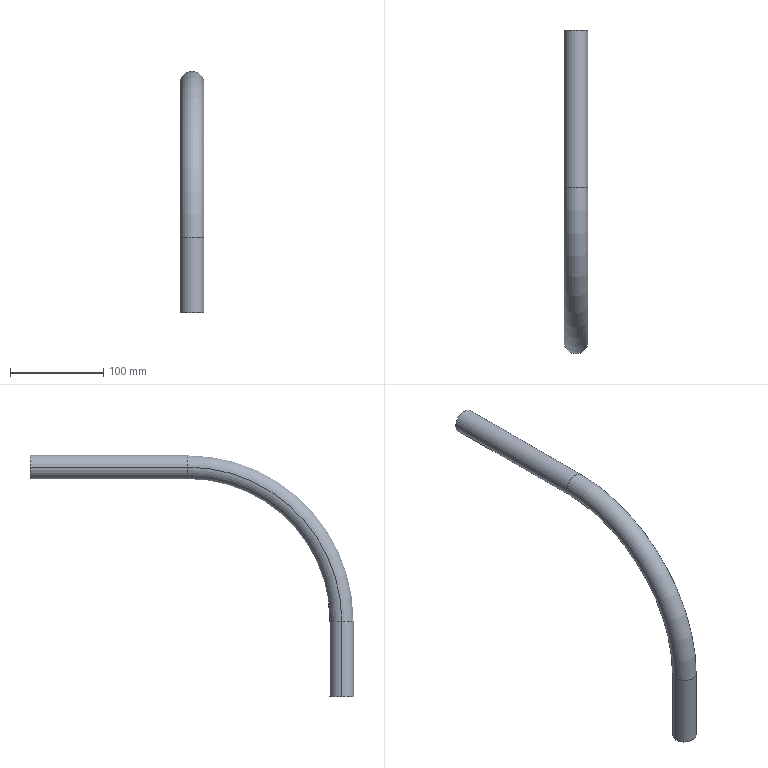Part | STEP file | 31E-01144WG10 | 1 solid | 17 faces | box 25.4 x 346.08 x 258.41 mm | volume 96204 mm3 | cylinder 10 | torus 4 | plane 3 | commonest cylinder face diameters 19.8 x4 25.4 x4 23 x2
STEP:
#1=CARTESIAN_POINT('',(-12.7,-168.38,0.));
#2=VERTEX_POINT('',#1);
#3=CARTESIAN_POINT('',(12.7,-168.38,0.));
#4=VERTEX_POINT('',#3);
#5=CARTESIAN_POINT('',(0.,-168.38,0.));
#6=DIRECTION('',(0.,1.,0.));
#7=AXIS2_PLACEMENT_3D('',#5,#6,$);
#8=CIRCLE('',#7,12.7);
#9=EDGE_CURVE('',#2,#4,#8,.T.);
#10=ORIENTED_EDGE('',*,*,#9,.T.);
#11=CARTESIAN_POINT('',(12.7,0.,0.));
#12=VERTEX_POINT('',#11);
#13=CARTESIAN_POINT('',(12.7,-84.19,0.));
#14=DIRECTION('',(0.,1.,0.));
#15=VECTOR('',#14,1.);
#16=LINE('',#13,#15);
#17=EDGE_CURVE('',#12,#4,#16,.F.);
#18=ORIENTED_EDGE('',*,*,#17,.F.);
#19=CARTESIAN_POINT('',(-12.7,0.,0.));
#20=VERTEX_POINT('',#19);
#21=CARTESIAN_POINT('',(0.,0.,0.));
#22=DIRECTION('',(0.,1.,0.));
#23=AXIS2_PLACEMENT_3D('',#21,#22,$);
#24=CIRCLE('',#23,12.7);
#25=EDGE_CURVE('',#20,#12,#24,.T.);
#26=ORIENTED_EDGE('',*,*,#25,.F.);
#27=CARTESIAN_POINT('',(-12.7,-84.19,0.));
#28=DIRECTION('',(0.,1.,0.));
#29=VECTOR('',#28,1.);
#30=LINE('',#27,#29);
#31=EDGE_CURVE('',#20,#2,#30,.F.);
#32=ORIENTED_EDGE('',*,*,#31,.T.);
#33=EDGE_LOOP('',(#10,#18,#26,#32));
#34=FACE_OUTER_BOUND('',#33,.T.);
#35=CARTESIAN_POINT('',(0.,-84.19,0.));
#36=DIRECTION('',(0.,1.,0.));
#37=DIRECTION('',(-1.,0.,0.));
#38=AXIS2_PLACEMENT_3D('',#35,#36,#37);
#39=CYLINDRICAL_SURFACE('',#38,12.7);
#40=ADVANCED_FACE('',(#34),#39,.T.);
#41=CARTESIAN_POINT('',(0.,-168.38,0.));
#42=DIRECTION('',(0.,1.,0.));
#43=AXIS2_PLACEMENT_3D('',#41,#42,$);
#44=CIRCLE('',#43,12.7);
#45=EDGE_CURVE('',#4,#2,#44,.T.);
#46=ORIENTED_EDGE('',*,*,#45,.T.);
#47=ORIENTED_EDGE('',*,*,#31,.F.);
#48=CARTESIAN_POINT('',(0.,0.,0.));
#49=DIRECTION('',(0.,1.,0.));
#50=AXIS2_PLACEMENT_3D('',#48,#49,$);
#51=CIRCLE('',#50,12.7);
#52=EDGE_CURVE('',#12,#20,#51,.T.);
#53=ORIENTED_EDGE('',*,*,#52,.F.);
#54=ORIENTED_EDGE('',*,*,#17,.T.);
#55=EDGE_LOOP('',(#46,#47,#53,#54));
#56=FACE_OUTER_BOUND('',#55,.T.);
#57=CARTESIAN_POINT('',(0.,-84.19,0.));
#58=DIRECTION('',(0.,1.,0.));
#59=DIRECTION('',(1.,0.,0.));
#60=AXIS2_PLACEMENT_3D('',#57,#58,#59);
#61=CYLINDRICAL_SURFACE('',#60,12.7);
#62=ADVANCED_FACE('',(#56),#61,.T.);
#63=CARTESIAN_POINT('',(-12.7,-333.38,-165.));
#64=VERTEX_POINT('',#63);
#65=CARTESIAN_POINT('',(12.7,-333.38,-165.));
#66=VERTEX_POINT('',#65);
#67=CARTESIAN_POINT('',(0.,-333.38,-165.));
#68=DIRECTION('',(0.,0.,1.));
#69=AXIS2_PLACEMENT_3D('',#67,#68,$);
#70=CIRCLE('',#69,12.7);
#71=EDGE_CURVE('',#64,#66,#70,.T.);
#72=ORIENTED_EDGE('',*,*,#71,.T.);
#73=CARTESIAN_POINT('',(12.7,-168.38,-165.));
#74=DIRECTION('',(1.,0.,0.));
#75=AXIS2_PLACEMENT_3D('',#73,#74,$);
#76=CIRCLE('',#75,165.);
#77=EDGE_CURVE('',#4,#66,#76,.T.);
#78=ORIENTED_EDGE('',*,*,#77,.F.);
#79=ORIENTED_EDGE('',*,*,#9,.F.);
#80=CARTESIAN_POINT('',(-12.7,-168.38,-165.));
#81=DIRECTION('',(1.,0.,0.));
#82=AXIS2_PLACEMENT_3D('',#80,#81,$);
#83=CIRCLE('',#82,165.);
#84=EDGE_CURVE('',#2,#64,#83,.T.);
#85=ORIENTED_EDGE('',*,*,#84,.T.);
#86=EDGE_LOOP('',(#72,#78,#79,#85));
#87=FACE_OUTER_BOUND('',#86,.T.);
#88=CARTESIAN_POINT('',(0.,-168.38,-165.));
#89=DIRECTION('',(1.,0.,0.));
#90=DIRECTION('',(0.,0.,1.));
#91=AXIS2_PLACEMENT_3D('',#88,#89,#90);
#92=TOROIDAL_SURFACE('',#91,165.,12.7);
#93=ADVANCED_FACE('',(#87),#92,.T.);
#94=CARTESIAN_POINT('',(0.,-333.38,-165.));
#95=DIRECTION('',(0.,0.,1.));
#96=AXIS2_PLACEMENT_3D('',#94,#95,$);
#97=CIRCLE('',#96,12.7);
#98=EDGE_CURVE('',#66,#64,#97,.T.);
#99=ORIENTED_EDGE('',*,*,#98,.T.);
#100=ORIENTED_EDGE('',*,*,#84,.F.);
#101=ORIENTED_EDGE('',*,*,#45,.F.);
#102=ORIENTED_EDGE('',*,*,#77,.T.);
#103=EDGE_LOOP('',(#99,#100,#101,#102));
#104=FACE_OUTER_BOUND('',#103,.T.);
#105=CARTESIAN_POINT('',(0.,-168.38,-165.));
#106=DIRECTION('',(1.,0.,0.));
#107=DIRECTION('',(0.,0.,1.));
#108=AXIS2_PLACEMENT_3D('',#105,#106,#107);
#109=TOROIDAL_SURFACE('',#108,165.,12.7);
#110=ADVANCED_FACE('',(#104),#109,.T.);
#111=CARTESIAN_POINT('',(-12.7,-333.38,-245.71));
#112=VERTEX_POINT('',#111);
#113=CARTESIAN_POINT('',(12.7,-333.38,-245.71));
#114=VERTEX_POINT('',#113);
#115=CARTESIAN_POINT('',(0.,-333.38,-245.71));
#116=DIRECTION('',(0.,0.,1.));
#117=AXIS2_PLACEMENT_3D('',#115,#116,$);
#118=CIRCLE('',#117,12.7);
#119=EDGE_CURVE('',#112,#114,#118,.T.);
#120=ORIENTED_EDGE('',*,*,#119,.T.);
#121=CARTESIAN_POINT('',(12.7,-333.38,-205.355));
#122=DIRECTION('',(0.,0.,1.));
#123=VECTOR('',#122,1.);
#124=LINE('',#121,#123);
#125=EDGE_CURVE('',#66,#114,#124,.F.);
#126=ORIENTED_EDGE('',*,*,#125,.F.);
#127=ORIENTED_EDGE('',*,*,#71,.F.);
#128=CARTESIAN_POINT('',(-12.7,-333.38,-205.355));
#129=DIRECTION('',(0.,0.,1.));
#130=VECTOR('',#129,1.);
#131=LINE('',#128,#130);
#132=EDGE_CURVE('',#64,#112,#131,.F.);
#133=ORIENTED_EDGE('',*,*,#132,.T.);
#134=EDGE_LOOP('',(#120,#126,#127,#133));
#135=FACE_OUTER_BOUND('',#134,.T.);
#136=CARTESIAN_POINT('',(0.,-333.38,-205.355));
#137=DIRECTION('',(0.,0.,1.));
#138=DIRECTION('',(-1.,0.,0.));
#139=AXIS2_PLACEMENT_3D('',#136,#137,#138);
#140=CYLINDRICAL_SURFACE('',#139,12.7);
#141=ADVANCED_FACE('',(#135),#140,.T.);
#142=CARTESIAN_POINT('',(0.,-333.38,-245.71));
#143=DIRECTION('',(0.,0.,1.));
#144=AXIS2_PLACEMENT_3D('',#142,#143,$);
#145=CIRCLE('',#144,12.7);
#146=EDGE_CURVE('',#114,#112,#145,.T.);
#147=ORIENTED_EDGE('',*,*,#146,.T.);
#148=ORIENTED_EDGE('',*,*,#132,.F.);
#149=ORIENTED_EDGE('',*,*,#98,.F.);
#150=ORIENTED_EDGE('',*,*,#125,.T.);
#151=EDGE_LOOP('',(#147,#148,#149,#150));
#152=FACE_OUTER_BOUND('',#151,.T.);
#153=CARTESIAN_POINT('',(0.,-333.38,-205.355));
#154=DIRECTION('',(0.,0.,1.));
#155=DIRECTION('',(1.,0.,0.));
#156=AXIS2_PLACEMENT_3D('',#153,#154,#155);
#157=CYLINDRICAL_SURFACE('',#156,12.7);
#158=ADVANCED_FACE('',(#152),#157,.T.);
#159=CARTESIAN_POINT('',(-9.9,-168.38,0.));
#160=VERTEX_POINT('',#159);
#161=CARTESIAN_POINT('',(-9.9,-333.38,-165.));
#162=VERTEX_POINT('',#161);
#163=CARTESIAN_POINT('',(-9.9,-168.38,-165.));
#164=DIRECTION('',(1.,0.,0.));
#165=AXIS2_PLACEMENT_3D('',#163,#164,$);
#166=CIRCLE('',#165,165.);
#167=EDGE_CURVE('',#160,#162,#166,.T.);
#168=ORIENTED_EDGE('',*,*,#167,.F.);
#169=CARTESIAN_POINT('',(9.9,-168.38,0.));
#170=VERTEX_POINT('',#169);
#171=CARTESIAN_POINT('',(0.,-168.38,0.));
#172=DIRECTION('',(0.,1.,0.));
#173=AXIS2_PLACEMENT_3D('',#171,#172,$);
#174=CIRCLE('',#173,9.9);
#175=EDGE_CURVE('',#160,#170,#174,.T.);
#176=ORIENTED_EDGE('',*,*,#175,.T.);
#177=CARTESIAN_POINT('',(9.9,-333.38,-165.));
#178=VERTEX_POINT('',#177);
#179=CARTESIAN_POINT('',(9.9,-168.38,-165.));
#180=DIRECTION('',(1.,0.,0.));
#181=AXIS2_PLACEMENT_3D('',#179,#180,$);
#182=CIRCLE('',#181,165.);
#183=EDGE_CURVE('',#170,#178,#182,.T.);
#184=ORIENTED_EDGE('',*,*,#183,.T.);
#185=CARTESIAN_POINT('',(0.,-333.38,-165.));
#186=DIRECTION('',(0.,0.,1.));
#187=AXIS2_PLACEMENT_3D('',#185,#186,$);
#188=CIRCLE('',#187,9.9);
#189=EDGE_CURVE('',#162,#178,#188,.T.);
#190=ORIENTED_EDGE('',*,*,#189,.F.);
#191=EDGE_LOOP('',(#168,#176,#184,#190));
#192=FACE_OUTER_BOUND('',#191,.T.);
#193=CARTESIAN_POINT('',(0.,-168.38,-165.));
#194=DIRECTION('',(1.,0.,0.));
#195=DIRECTION('',(0.,0.,1.));
#196=AXIS2_PLACEMENT_3D('',#193,#194,#195);
#197=TOROIDAL_SURFACE('',#196,165.,9.9);
#198=ADVANCED_FACE('',(#192),#197,.F.);
#199=ORIENTED_EDGE('',*,*,#183,.F.);
#200=CARTESIAN_POINT('',(0.,-168.38,0.));
#201=DIRECTION('',(0.,1.,0.));
#202=AXIS2_PLACEMENT_3D('',#200,#201,$);
#203=CIRCLE('',#202,9.9);
#204=EDGE_CURVE('',#170,#160,#203,.T.);
#205=ORIENTED_EDGE('',*,*,#204,.T.);
#206=ORIENTED_EDGE('',*,*,#167,.T.);
#207=CARTESIAN_POINT('',(0.,-333.38,-165.));
#208=DIRECTION('',(0.,0.,1.));
#209=AXIS2_PLACEMENT_3D('',#207,#208,$);
#210=CIRCLE('',#209,9.9);
#211=EDGE_CURVE('',#178,#162,#210,.T.);
#212=ORIENTED_EDGE('',*,*,#211,.F.);
#213=EDGE_LOOP('',(#199,#205,#206,#212));
#214=FACE_OUTER_BOUND('',#213,.T.);
#215=CARTESIAN_POINT('',(0.,-168.38,-165.));
#216=DIRECTION('',(1.,0.,0.));
#217=DIRECTION('',(0.,0.,1.));
#218=AXIS2_PLACEMENT_3D('',#215,#216,#217);
#219=TOROIDAL_SURFACE('',#218,165.,9.9);
#220=ADVANCED_FACE('',(#214),#219,.F.);
#221=ORIENTED_EDGE('',*,*,#146,.F.);
#222=ORIENTED_EDGE('',*,*,#119,.F.);
#223=EDGE_LOOP('',(#221,#222));
#224=FACE_OUTER_BOUND('',#223,.T.);
#225=CARTESIAN_POINT('',(9.9,-333.38,-245.71));
#226=VERTEX_POINT('',#225);
#227=CARTESIAN_POINT('',(-9.9,-333.38,-245.71));
#228=VERTEX_POINT('',#227);
#229=CARTESIAN_POINT('',(0.,-333.38,-245.71));
#230=DIRECTION('',(0.,0.,-1.));
#231=AXIS2_PLACEMENT_3D('',#229,#230,$);
#232=CIRCLE('',#231,9.9);
#233=EDGE_CURVE('',#226,#228,#232,.F.);
#234=ORIENTED_EDGE('',*,*,#233,.T.);
#235=CARTESIAN_POINT('',(0.,-333.38,-245.71));
#236=DIRECTION('',(0.,0.,-1.));
#237=AXIS2_PLACEMENT_3D('',#235,#236,$);
#238=CIRCLE('',#237,9.9);
#239=EDGE_CURVE('',#228,#226,#238,.F.);
#240=ORIENTED_EDGE('',*,*,#239,.T.);
#241=EDGE_LOOP('',(#234,#240));
#242=FACE_BOUND('',#241,.T.);
#243=CARTESIAN_POINT('',(0.,-333.38,-245.71));
#244=DIRECTION('',(0.,0.,-1.));
#245=DIRECTION('',(0.,1.,0.));
#246=AXIS2_PLACEMENT_3D('',#243,#244,#245);
#247=PLANE('',#246);
#248=ADVANCED_FACE('',(#224,#242),#247,.T.);
#249=CARTESIAN_POINT('',(-9.9,-333.38,-205.355));
#250=DIRECTION('',(0.,0.,1.));
#251=VECTOR('',#250,1.);
#252=LINE('',#249,#251);
#253=EDGE_CURVE('',#162,#228,#252,.F.);
#254=ORIENTED_EDGE('',*,*,#253,.F.);
#255=ORIENTED_EDGE('',*,*,#189,.T.);
#256=CARTESIAN_POINT('',(9.9,-333.38,-205.355));
#257=DIRECTION('',(0.,0.,1.));
#258=VECTOR('',#257,1.);
#259=LINE('',#256,#258);
#260=EDGE_CURVE('',#178,#226,#259,.F.);
#261=ORIENTED_EDGE('',*,*,#260,.T.);
#262=ORIENTED_EDGE('',*,*,#239,.F.);
#263=EDGE_LOOP('',(#254,#255,#261,#262));
#264=FACE_OUTER_BOUND('',#263,.T.);
#265=CARTESIAN_POINT('',(0.,-333.38,-205.355));
#266=DIRECTION('',(0.,0.,1.));
#267=DIRECTION('',(-1.,0.,0.));
#268=AXIS2_PLACEMENT_3D('',#265,#266,#267);
#269=CYLINDRICAL_SURFACE('',#268,9.9);
#270=ADVANCED_FACE('',(#264),#269,.F.);
#271=ORIENTED_EDGE('',*,*,#260,.F.);
#272=ORIENTED_EDGE('',*,*,#211,.T.);
#273=ORIENTED_EDGE('',*,*,#253,.T.);
#274=ORIENTED_EDGE('',*,*,#233,.F.);
#275=EDGE_LOOP('',(#271,#272,#273,#274));
#276=FACE_OUTER_BOUND('',#275,.T.);
#277=CARTESIAN_POINT('',(0.,-333.38,-205.355));
#278=DIRECTION('',(0.,0.,1.));
#279=DIRECTION('',(1.,0.,0.));
#280=AXIS2_PLACEMENT_3D('',#277,#278,#279);
#281=CYLINDRICAL_SURFACE('',#280,9.9);
#282=ADVANCED_FACE('',(#276),#281,.F.);
#283=CARTESIAN_POINT('',(9.9,-45.,0.));
#284=VERTEX_POINT('',#283);
#285=CARTESIAN_POINT('',(-9.9,-45.,0.));
#286=VERTEX_POINT('',#285);
#287=CARTESIAN_POINT('',(0.,-45.,0.));
#288=DIRECTION('',(0.,1.,0.));
#289=AXIS2_PLACEMENT_3D('',#287,#288,$);
#290=CIRCLE('',#289,9.9);
#291=EDGE_CURVE('',#284,#286,#290,.T.);
#292=ORIENTED_EDGE('',*,*,#291,.T.);
#293=CARTESIAN_POINT('',(-9.9,-84.19,0.));
#294=DIRECTION('',(0.,1.,0.));
#295=VECTOR('',#294,1.);
#296=LINE('',#293,#295);
#297=EDGE_CURVE('',#286,#160,#296,.F.);
#298=ORIENTED_EDGE('',*,*,#297,.T.);
#299=ORIENTED_EDGE('',*,*,#204,.F.);
#300=CARTESIAN_POINT('',(9.9,-84.19,0.));
#301=DIRECTION('',(0.,1.,0.));
#302=VECTOR('',#301,1.);
#303=LINE('',#300,#302);
#304=EDGE_CURVE('',#284,#170,#303,.F.);
#305=ORIENTED_EDGE('',*,*,#304,.F.);
#306=EDGE_LOOP('',(#292,#298,#299,#305));
#307=FACE_OUTER_BOUND('',#306,.T.);
#308=CARTESIAN_POINT('',(0.,-84.19,0.));
#309=DIRECTION('',(0.,1.,0.));
#310=DIRECTION('',(1.,0.,0.));
#311=AXIS2_PLACEMENT_3D('',#308,#309,#310);
#312=CYLINDRICAL_SURFACE('',#311,9.9);
#313=ADVANCED_FACE('',(#307),#312,.F.);
#314=CARTESIAN_POINT('',(0.,-45.,0.));
#315=DIRECTION('',(0.,1.,0.));
#316=AXIS2_PLACEMENT_3D('',#314,#315,$);
#317=CIRCLE('',#316,9.9);
#318=EDGE_CURVE('',#286,#284,#317,.T.);
#319=ORIENTED_EDGE('',*,*,#318,.T.);
#320=ORIENTED_EDGE('',*,*,#304,.T.);
#321=ORIENTED_EDGE('',*,*,#175,.F.);
#322=ORIENTED_EDGE('',*,*,#297,.F.);
#323=EDGE_LOOP('',(#319,#320,#321,#322));
#324=FACE_OUTER_BOUND('',#323,.T.);
#325=CARTESIAN_POINT('',(0.,-84.19,0.));
#326=DIRECTION('',(0.,1.,0.));
#327=DIRECTION('',(-1.,0.,0.));
#328=AXIS2_PLACEMENT_3D('',#325,#326,#327);
#329=CYLINDRICAL_SURFACE('',#328,9.9);
#330=ADVANCED_FACE('',(#324),#329,.F.);
#331=ORIENTED_EDGE('',*,*,#25,.T.);
#332=ORIENTED_EDGE('',*,*,#52,.T.);
#333=EDGE_LOOP('',(#331,#332));
#334=FACE_OUTER_BOUND('',#333,.T.);
#335=CARTESIAN_POINT('',(-11.5,0.,0.));
#336=VERTEX_POINT('',#335);
#337=CARTESIAN_POINT('',(11.5,0.,0.));
#338=VERTEX_POINT('',#337);
#339=CARTESIAN_POINT('',(0.,0.,0.));
#340=DIRECTION('',(0.,1.,0.));
#341=AXIS2_PLACEMENT_3D('',#339,#340,$);
#342=CIRCLE('',#341,11.5);
#343=EDGE_CURVE('',#336,#338,#342,.T.);
#344=ORIENTED_EDGE('',*,*,#343,.F.);
#345=CARTESIAN_POINT('',(0.,0.,0.));
#346=DIRECTION('',(0.,1.,0.));
#347=AXIS2_PLACEMENT_3D('',#345,#346,$);
#348=CIRCLE('',#347,11.5);
#349=EDGE_CURVE('',#338,#336,#348,.T.);
#350=ORIENTED_EDGE('',*,*,#349,.F.);
#351=EDGE_LOOP('',(#344,#350));
#352=FACE_BOUND('',#351,.T.);
#353=CARTESIAN_POINT('',(0.,0.,0.));
#354=DIRECTION('',(0.,1.,0.));
#355=DIRECTION('',(0.,0.,1.));
#356=AXIS2_PLACEMENT_3D('',#353,#354,#355);
#357=PLANE('',#356);
#358=ADVANCED_FACE('',(#334,#352),#357,.T.);
#359=CARTESIAN_POINT('',(-11.5,-45.,0.));
#360=VERTEX_POINT('',#359);
#361=CARTESIAN_POINT('',(-11.5,-22.5,0.));
#362=DIRECTION('',(0.,1.,0.));
#363=VECTOR('',#362,1.);
#364=LINE('',#361,#363);
#365=EDGE_CURVE('',#336,#360,#364,.F.);
#366=ORIENTED_EDGE('',*,*,#365,.F.);
#367=ORIENTED_EDGE('',*,*,#343,.T.);
#368=CARTESIAN_POINT('',(11.5,-45.,0.));
#369=VERTEX_POINT('',#368);
#370=CARTESIAN_POINT('',(11.5,-22.5,0.));
#371=DIRECTION('',(0.,1.,0.));
#372=VECTOR('',#371,1.);
#373=LINE('',#370,#372);
#374=EDGE_CURVE('',#338,#369,#373,.F.);
#375=ORIENTED_EDGE('',*,*,#374,.T.);
#376=CARTESIAN_POINT('',(0.,-45.,0.));
#377=DIRECTION('',(0.,1.,0.));
#378=AXIS2_PLACEMENT_3D('',#376,#377,$);
#379=CIRCLE('',#378,11.5);
#380=EDGE_CURVE('',#360,#369,#379,.T.);
#381=ORIENTED_EDGE('',*,*,#380,.F.);
#382=EDGE_LOOP('',(#366,#367,#375,#381));
#383=FACE_OUTER_BOUND('',#382,.T.);
#384=CARTESIAN_POINT('',(0.,-22.5,0.));
#385=DIRECTION('',(0.,1.,0.));
#386=DIRECTION('',(-1.,0.,0.));
#387=AXIS2_PLACEMENT_3D('',#384,#385,#386);
#388=CYLINDRICAL_SURFACE('',#387,11.5);
#389=ADVANCED_FACE('',(#383),#388,.F.);
#390=ORIENTED_EDGE('',*,*,#374,.F.);
#391=ORIENTED_EDGE('',*,*,#349,.T.);
#392=ORIENTED_EDGE('',*,*,#365,.T.);
#393=CARTESIAN_POINT('',(0.,-45.,0.));
#394=DIRECTION('',(0.,1.,0.));
#395=AXIS2_PLACEMENT_3D('',#393,#394,$);
#396=CIRCLE('',#395,11.5);
#397=EDGE_CURVE('',#369,#360,#396,.T.);
#398=ORIENTED_EDGE('',*,*,#397,.F.);
#399=EDGE_LOOP('',(#390,#391,#392,#398));
#400=FACE_OUTER_BOUND('',#399,.T.);
#401=ADVANCED_FACE('',(#400),#388,.F.);
#402=ORIENTED_EDGE('',*,*,#380,.T.);
#403=ORIENTED_EDGE('',*,*,#397,.T.);
#404=EDGE_LOOP('',(#402,#403));
#405=FACE_OUTER_BOUND('',#404,.T.);
#406=ORIENTED_EDGE('',*,*,#318,.F.);
#407=ORIENTED_EDGE('',*,*,#291,.F.);
#408=EDGE_LOOP('',(#406,#407));
#409=FACE_BOUND('',#408,.T.);
#410=CARTESIAN_POINT('',(0.,-45.,0.));
#411=DIRECTION('',(0.,1.,0.));
#412=DIRECTION('',(-1.,0.,0.));
#413=AXIS2_PLACEMENT_3D('',#410,#411,#412);
#414=PLANE('',#413);
#415=ADVANCED_FACE('',(#405,#409),#414,.T.);
#416=CLOSED_SHELL('',(#40,#62,#93,#110,#141,#158,#198,#220,#248,#270,#282,#313,#330,#358,#389,#401,#415));
#417=MANIFOLD_SOLID_BREP('',#416);
#418=(LENGTH_UNIT()NAMED_UNIT(*)SI_UNIT(.MILLI.,.METRE.));
#419=UNCERTAINTY_MEASURE_WITH_UNIT(LENGTH_MEASURE(0.005),#418,'','');
#420=(NAMED_UNIT(*)PLANE_ANGLE_UNIT()SI_UNIT($,.RADIAN.));
#421=(NAMED_UNIT(*)SI_UNIT($,.STERADIAN.)SOLID_ANGLE_UNIT());
#422=(GEOMETRIC_REPRESENTATION_CONTEXT(3)GLOBAL_UNCERTAINTY_ASSIGNED_CONTEXT((#419))GLOBAL_UNIT_ASSIGNED_CONTEXT((#418,#420,#421))REPRESENTATION_CONTEXT('',''));
#423=ADVANCED_BREP_SHAPE_REPRESENTATION('',(#417),#422);